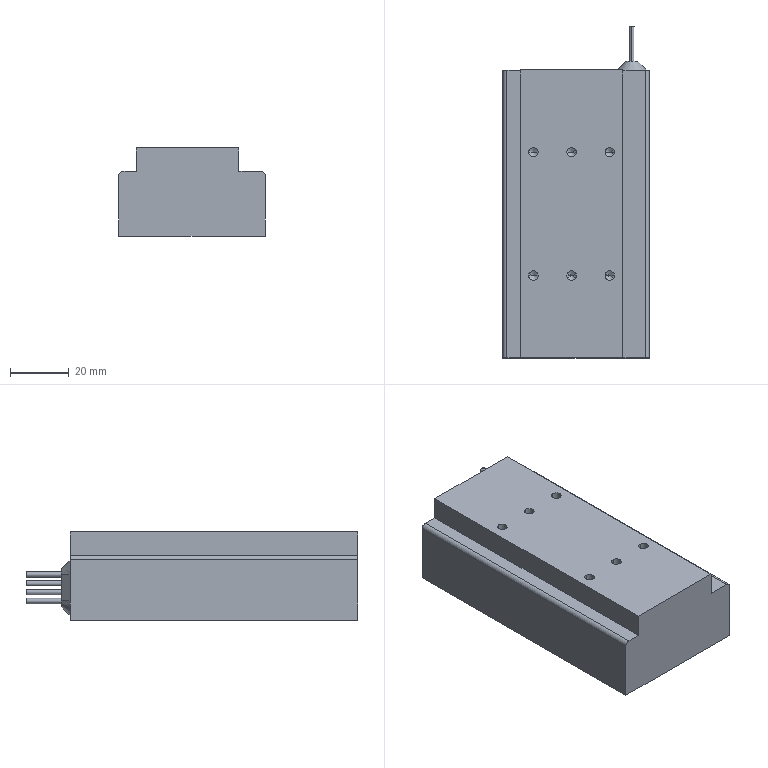Part | STEP file | 1 solid | 62 faces | box 50 x 113 x 30 mm | volume 135231 mm3 | cylinder 26 | cone 19 | plane 17 | commonest cylinder face diameters 3.242 x12 1.8 x8 2.459 x4 3 x2